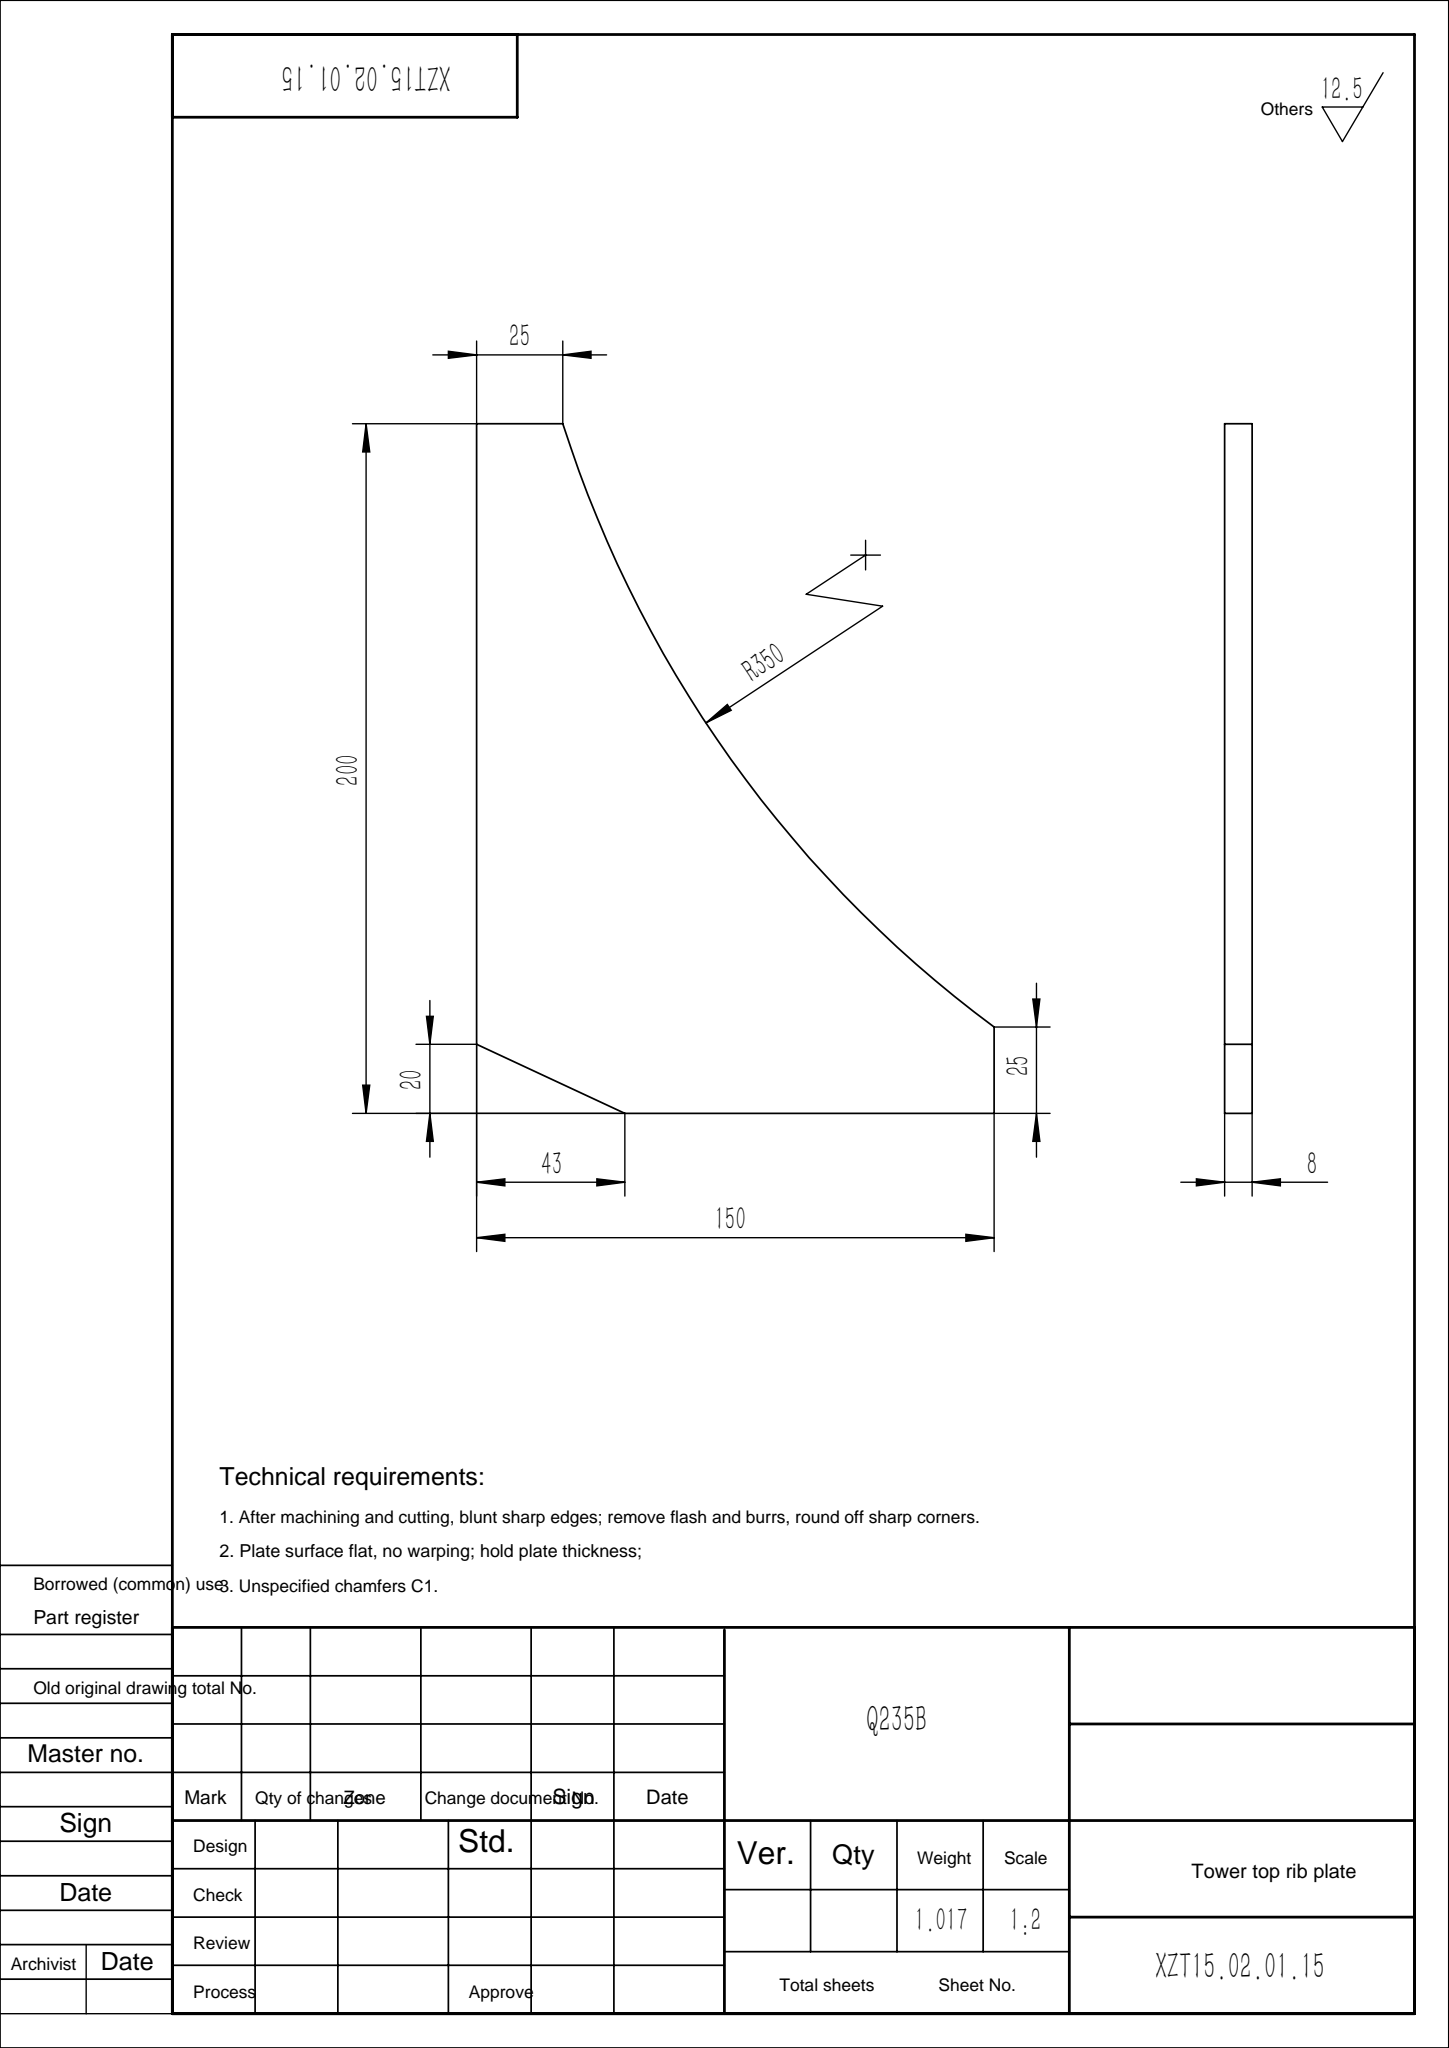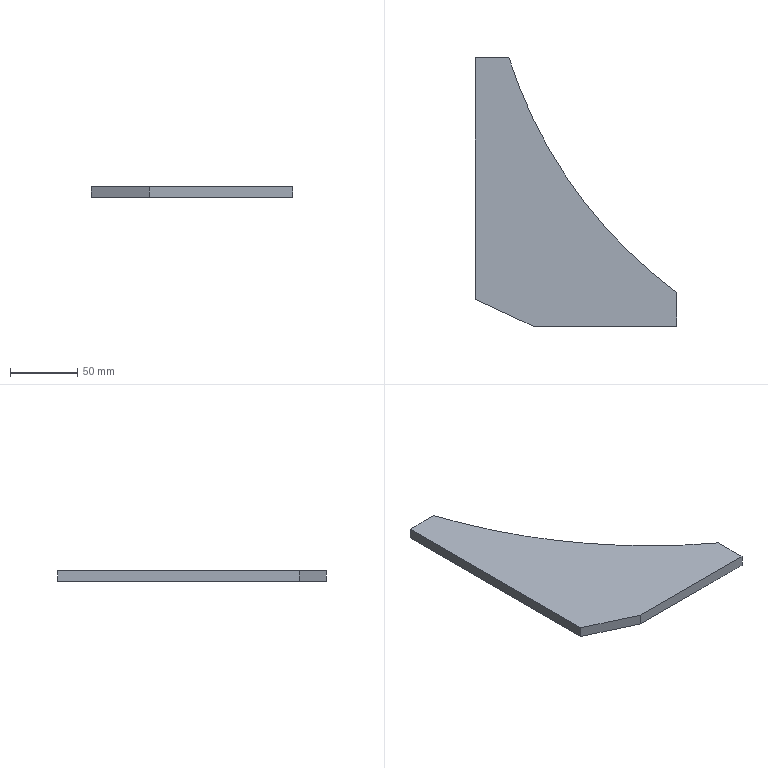Part | SolidWorks | features Chamfer 1, Extrusion 1, ICE 1 | 1 solid | 8 faces | box 150 x 200 x 8 mm | volume 129549 mm3 | plane 7 | cylinder 1 | commonest cylinder face diameters 700 x1
STEP:
#1=CARTESIAN_POINT('',(0.,200.,-4.));
#2=VERTEX_POINT('',#1);
#3=CARTESIAN_POINT('',(0.,20.,-4.));
#4=VERTEX_POINT('',#3);
#5=CARTESIAN_POINT('',(0.,200.,-4.));
#6=DIRECTION('',(0.,-1.,0.));
#7=VECTOR('',#6,1000.);
#8=LINE('',#5,#7);
#9=EDGE_CURVE('',#2,#4,#8,.T.);
#10=ORIENTED_EDGE('',*,*,#9,.T.);
#11=CARTESIAN_POINT('',(0.,20.,4.));
#12=VERTEX_POINT('',#11);
#13=CARTESIAN_POINT('',(0.,20.,4.));
#14=DIRECTION('',(0.,0.,1.));
#15=VECTOR('',#14,1000.);
#16=LINE('',#13,#15);
#17=EDGE_CURVE('',#4,#12,#16,.T.);
#18=ORIENTED_EDGE('',*,*,#17,.T.);
#19=CARTESIAN_POINT('',(0.,200.,4.));
#20=VERTEX_POINT('',#19);
#21=CARTESIAN_POINT('',(0.,200.,4.));
#22=DIRECTION('',(0.,-1.,0.));
#23=VECTOR('',#22,1000.);
#24=LINE('',#21,#23);
#25=EDGE_CURVE('',#20,#12,#24,.T.);
#26=ORIENTED_EDGE('',*,*,#25,.F.);
#27=CARTESIAN_POINT('',(0.,200.,4.));
#28=DIRECTION('',(0.,0.,-1.));
#29=VECTOR('',#28,1000.);
#30=LINE('',#27,#29);
#31=EDGE_CURVE('',#20,#2,#30,.T.);
#32=ORIENTED_EDGE('',*,*,#31,.T.);
#33=EDGE_LOOP('',(#10,#18,#26,#32));
#34=FACE_OUTER_BOUND('',#33,.T.);
#35=CARTESIAN_POINT('',(0.,200.,4.));
#36=DIRECTION('',(1.,0.,0.));
#37=DIRECTION('',(0.,1.,0.));
#38=AXIS2_PLACEMENT_3D('',#35,#36,#37);
#39=PLANE('',#38);
#40=ADVANCED_FACE('',(#34),#39,.F.);
#41=CARTESIAN_POINT('',(43.,0.,4.));
#42=VERTEX_POINT('',#41);
#43=CARTESIAN_POINT('',(150.,0.,4.));
#44=VERTEX_POINT('',#43);
#45=CARTESIAN_POINT('',(0.,0.,4.));
#46=DIRECTION('',(1.,0.,0.));
#47=VECTOR('',#46,1000.);
#48=LINE('',#45,#47);
#49=EDGE_CURVE('',#42,#44,#48,.T.);
#50=ORIENTED_EDGE('',*,*,#49,.F.);
#51=CARTESIAN_POINT('',(43.,0.,-4.));
#52=VERTEX_POINT('',#51);
#53=CARTESIAN_POINT('',(43.,0.,4.));
#54=DIRECTION('',(0.,0.,-1.));
#55=VECTOR('',#54,1000.);
#56=LINE('',#53,#55);
#57=EDGE_CURVE('',#42,#52,#56,.T.);
#58=ORIENTED_EDGE('',*,*,#57,.T.);
#59=CARTESIAN_POINT('',(150.,0.,-4.));
#60=VERTEX_POINT('',#59);
#61=CARTESIAN_POINT('',(0.,0.,-4.));
#62=DIRECTION('',(1.,0.,0.));
#63=VECTOR('',#62,1000.);
#64=LINE('',#61,#63);
#65=EDGE_CURVE('',#52,#60,#64,.T.);
#66=ORIENTED_EDGE('',*,*,#65,.T.);
#67=CARTESIAN_POINT('',(150.,0.,4.));
#68=DIRECTION('',(0.,0.,-1.));
#69=VECTOR('',#68,1000.);
#70=LINE('',#67,#69);
#71=EDGE_CURVE('',#44,#60,#70,.T.);
#72=ORIENTED_EDGE('',*,*,#71,.F.);
#73=EDGE_LOOP('',(#50,#58,#66,#72));
#74=FACE_OUTER_BOUND('',#73,.T.);
#75=CARTESIAN_POINT('',(0.,0.,4.));
#76=DIRECTION('',(0.,1.,0.));
#77=DIRECTION('',(0.,0.,1.));
#78=AXIS2_PLACEMENT_3D('',#75,#76,#77);
#79=PLANE('',#78);
#80=ADVANCED_FACE('',(#74),#79,.F.);
#81=CARTESIAN_POINT('',(150.,25.,-4.));
#82=VERTEX_POINT('',#81);
#83=CARTESIAN_POINT('',(150.,0.,-4.));
#84=DIRECTION('',(0.,1.,0.));
#85=VECTOR('',#84,1000.);
#86=LINE('',#83,#85);
#87=EDGE_CURVE('',#60,#82,#86,.T.);
#88=ORIENTED_EDGE('',*,*,#87,.T.);
#89=CARTESIAN_POINT('',(150.,25.,4.));
#90=VERTEX_POINT('',#89);
#91=CARTESIAN_POINT('',(150.,25.,4.));
#92=DIRECTION('',(0.,0.,-1.));
#93=VECTOR('',#92,1000.);
#94=LINE('',#91,#93);
#95=EDGE_CURVE('',#90,#82,#94,.T.);
#96=ORIENTED_EDGE('',*,*,#95,.F.);
#97=CARTESIAN_POINT('',(150.,0.,4.));
#98=DIRECTION('',(0.,1.,0.));
#99=VECTOR('',#98,1000.);
#100=LINE('',#97,#99);
#101=EDGE_CURVE('',#44,#90,#100,.T.);
#102=ORIENTED_EDGE('',*,*,#101,.F.);
#103=ORIENTED_EDGE('',*,*,#71,.T.);
#104=EDGE_LOOP('',(#88,#96,#102,#103));
#105=FACE_OUTER_BOUND('',#104,.T.);
#106=CARTESIAN_POINT('',(150.,0.,4.));
#107=DIRECTION('',(-1.,0.,0.));
#108=DIRECTION('',(0.,0.,1.));
#109=AXIS2_PLACEMENT_3D('',#106,#107,#108);
#110=PLANE('',#109);
#111=ADVANCED_FACE('',(#105),#110,.F.);
#112=CARTESIAN_POINT('',(25.,200.,-4.));
#113=VERTEX_POINT('',#112);
#114=CARTESIAN_POINT('',(25.,200.,-4.));
#115=DIRECTION('',(-1.,0.,0.));
#116=VECTOR('',#115,1000.);
#117=LINE('',#114,#116);
#118=EDGE_CURVE('',#113,#2,#117,.T.);
#119=ORIENTED_EDGE('',*,*,#118,.T.);
#120=ORIENTED_EDGE('',*,*,#31,.F.);
#121=CARTESIAN_POINT('',(25.,200.,4.));
#122=VERTEX_POINT('',#121);
#123=CARTESIAN_POINT('',(25.,200.,4.));
#124=DIRECTION('',(-1.,0.,0.));
#125=VECTOR('',#124,1000.);
#126=LINE('',#123,#125);
#127=EDGE_CURVE('',#122,#20,#126,.T.);
#128=ORIENTED_EDGE('',*,*,#127,.F.);
#129=CARTESIAN_POINT('',(25.,200.,4.));
#130=DIRECTION('',(0.,0.,-1.));
#131=VECTOR('',#130,1000.);
#132=LINE('',#129,#131);
#133=EDGE_CURVE('',#122,#113,#132,.T.);
#134=ORIENTED_EDGE('',*,*,#133,.T.);
#135=EDGE_LOOP('',(#119,#120,#128,#134));
#136=FACE_OUTER_BOUND('',#135,.T.);
#137=CARTESIAN_POINT('',(25.,200.,4.));
#138=DIRECTION('',(0.,-1.,0.));
#139=DIRECTION('',(0.,0.,-1.));
#140=AXIS2_PLACEMENT_3D('',#137,#138,#139);
#141=PLANE('',#140);
#142=ADVANCED_FACE('',(#136),#141,.F.);
#143=CARTESIAN_POINT('',(358.532,306.095,4.));
#144=DIRECTION('',(0.,0.,1.));
#145=DIRECTION('',(1.,0.,0.));
#146=AXIS2_PLACEMENT_3D('',#143,#144,#145);
#147=CIRCLE('',#146,350.);
#148=EDGE_CURVE('',#122,#90,#147,.T.);
#149=ORIENTED_EDGE('',*,*,#148,.F.);
#150=ORIENTED_EDGE('',*,*,#127,.T.);
#151=ORIENTED_EDGE('',*,*,#25,.T.);
#152=CARTESIAN_POINT('',(7.648,16.443,4.));
#153=DIRECTION('',(0.9067,-0.4217,0.));
#154=VECTOR('',#153,1000.);
#155=LINE('',#152,#154);
#156=EDGE_CURVE('',#12,#42,#155,.T.);
#157=ORIENTED_EDGE('',*,*,#156,.T.);
#158=ORIENTED_EDGE('',*,*,#49,.T.);
#159=ORIENTED_EDGE('',*,*,#101,.T.);
#160=EDGE_LOOP('',(#149,#150,#151,#157,#158,#159));
#161=FACE_OUTER_BOUND('',#160,.T.);
#162=CARTESIAN_POINT('',(0.,0.,4.));
#163=DIRECTION('',(0.,0.,1.));
#164=DIRECTION('',(1.,0.,0.));
#165=AXIS2_PLACEMENT_3D('',#162,#163,#164);
#166=PLANE('',#165);
#167=ADVANCED_FACE('',(#161),#166,.T.);
#168=ORIENTED_EDGE('',*,*,#118,.F.);
#169=CARTESIAN_POINT('',(358.532,306.095,-4.));
#170=DIRECTION('',(0.,0.,1.));
#171=DIRECTION('',(1.,0.,0.));
#172=AXIS2_PLACEMENT_3D('',#169,#170,#171);
#173=CIRCLE('',#172,350.);
#174=EDGE_CURVE('',#113,#82,#173,.T.);
#175=ORIENTED_EDGE('',*,*,#174,.T.);
#176=ORIENTED_EDGE('',*,*,#87,.F.);
#177=ORIENTED_EDGE('',*,*,#65,.F.);
#178=CARTESIAN_POINT('',(43.,0.,-4.));
#179=DIRECTION('',(-0.9067,0.4217,0.));
#180=VECTOR('',#179,1000.);
#181=LINE('',#178,#180);
#182=EDGE_CURVE('',#52,#4,#181,.T.);
#183=ORIENTED_EDGE('',*,*,#182,.T.);
#184=ORIENTED_EDGE('',*,*,#9,.F.);
#185=EDGE_LOOP('',(#168,#175,#176,#177,#183,#184));
#186=FACE_OUTER_BOUND('',#185,.T.);
#187=CARTESIAN_POINT('',(0.,0.,-4.));
#188=DIRECTION('',(0.,0.,1.));
#189=DIRECTION('',(1.,0.,0.));
#190=AXIS2_PLACEMENT_3D('',#187,#188,#189);
#191=PLANE('',#190);
#192=ADVANCED_FACE('',(#186),#191,.F.);
#193=ORIENTED_EDGE('',*,*,#156,.F.);
#194=ORIENTED_EDGE('',*,*,#17,.F.);
#195=ORIENTED_EDGE('',*,*,#182,.F.);
#196=ORIENTED_EDGE('',*,*,#57,.F.);
#197=EDGE_LOOP('',(#193,#194,#195,#196));
#198=FACE_OUTER_BOUND('',#197,.T.);
#199=CARTESIAN_POINT('',(43.,0.,4.));
#200=DIRECTION('',(0.4217,0.9067,0.));
#201=DIRECTION('',(0.,0.,-1.));
#202=AXIS2_PLACEMENT_3D('',#199,#200,#201);
#203=PLANE('',#202);
#204=ADVANCED_FACE('',(#198),#203,.F.);
#205=ORIENTED_EDGE('',*,*,#133,.F.);
#206=ORIENTED_EDGE('',*,*,#148,.T.);
#207=ORIENTED_EDGE('',*,*,#95,.T.);
#208=ORIENTED_EDGE('',*,*,#174,.F.);
#209=EDGE_LOOP('',(#205,#206,#207,#208));
#210=FACE_OUTER_BOUND('',#209,.T.);
#211=CARTESIAN_POINT('',(358.532,306.095,-6.));
#212=DIRECTION('',(0.,0.,1.));
#213=DIRECTION('',(1.,0.,0.));
#214=AXIS2_PLACEMENT_3D('',#211,#212,#213);
#215=CYLINDRICAL_SURFACE('',#214,350.);
#216=ADVANCED_FACE('',(#210),#215,.F.);
#217=CLOSED_SHELL('',(#40,#80,#111,#142,#167,#192,#204,#216));
#218=MANIFOLD_SOLID_BREP('',#217);
#219=CARTESIAN_POINT('',(0.,0.,0.));
#220=DIRECTION('',(0.,0.,1.));
#221=DIRECTION('',(1.,0.,0.));
#222=AXIS2_PLACEMENT_3D('',#219,#220,#221);
#223=(LENGTH_UNIT()NAMED_UNIT(*)SI_UNIT(.MILLI.,.METRE.));
#224=UNCERTAINTY_MEASURE_WITH_UNIT(LENGTH_MEASURE(0.00001),#223,'','');
#225=(NAMED_UNIT(*)PLANE_ANGLE_UNIT()SI_UNIT($,.RADIAN.));
#226=(NAMED_UNIT(*)SI_UNIT($,.STERADIAN.)SOLID_ANGLE_UNIT());
#227=(GEOMETRIC_REPRESENTATION_CONTEXT(3)GLOBAL_UNCERTAINTY_ASSIGNED_CONTEXT((#224))GLOBAL_UNIT_ASSIGNED_CONTEXT((#223,#225,#226))REPRESENTATION_CONTEXT('',''));
#228=ADVANCED_BREP_SHAPE_REPRESENTATION('',(#218,#222),#227);